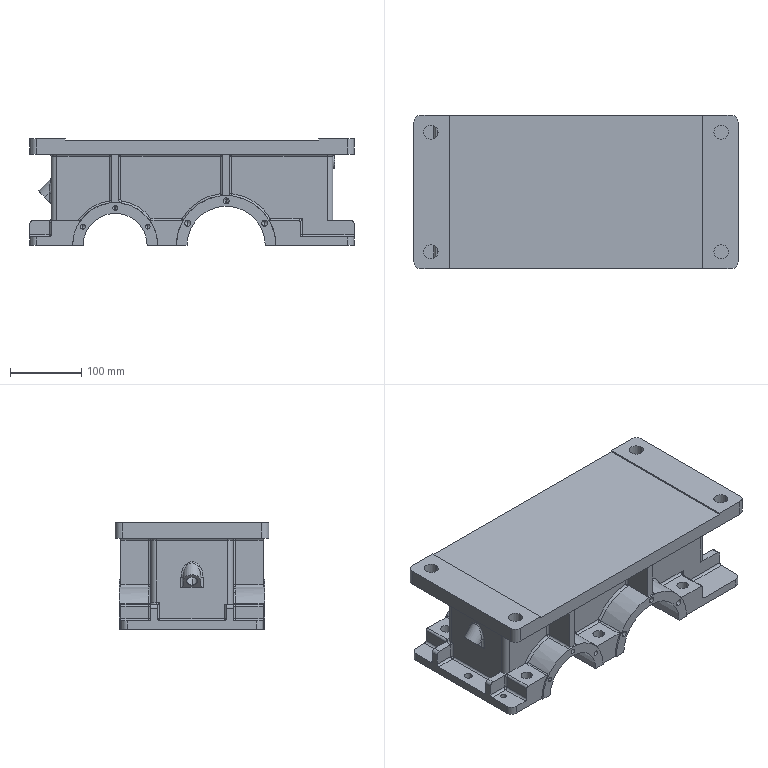Part | SolidWorks | features Fillet 25, ICE 15, 3DProfileFeature 4, HoleWzd 4, Chamfer 1, Extrusion 1, MirrorPattern 1, Sweep 1 | 1 solid | 340 faces | box 456 x 216 x 150 mm | volume 3465010 mm3 | cylinder 177 | plane 84 | sphere 33 | cone 26 | torus 17 | spline 3 | commonest cylinder face diameters 6 x81 20 x18 16 x16 6.8 x12 8.5 x12 32 x8